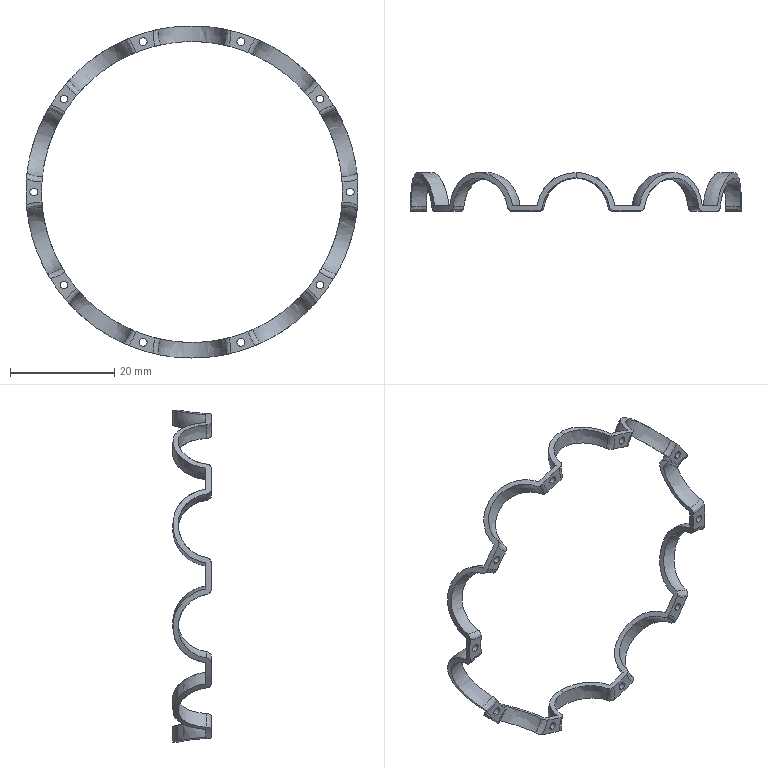Part | STEP file | Case | 1 solid | 84 faces | box 63.56 x 7.5 x 63.56 mm | volume 756.109 mm3 | spline 40 | cylinder 24 | plane 20 | commonest cylinder face diameters 1.5 x20 57.56 x2 63.56 x2